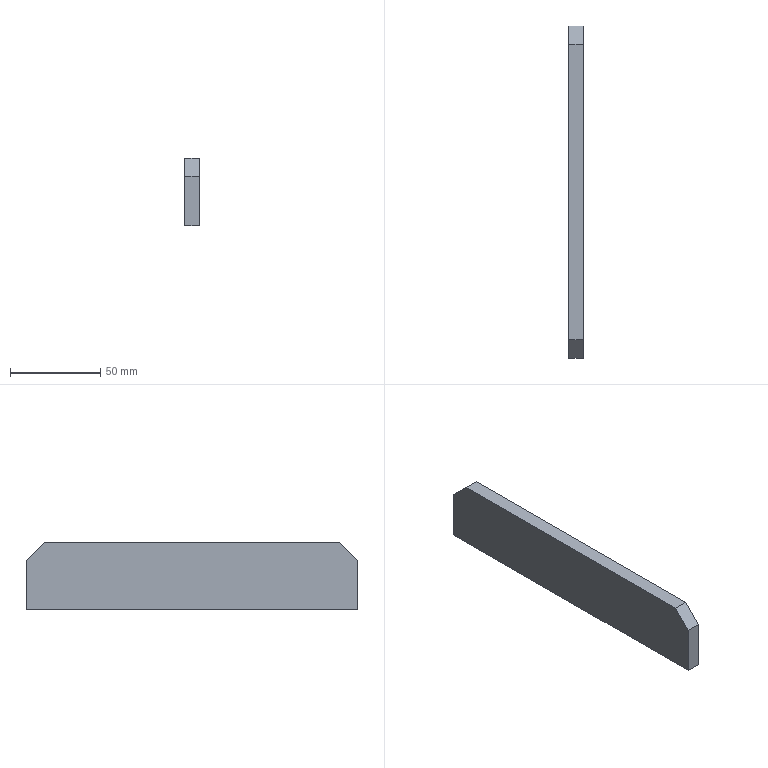Part | STEP file | Beam填充筋Plate-200×100 | 1 solid | 8 faces | box 8 x 184 x 37.25 mm | volume 54032 mm3 | plane 8
STEP:
#1=CARTESIAN_POINT('',(0.,0.,0.));
#2=DIRECTION('',(0.,0.,1.));
#3=DIRECTION('',(1.,0.,0.));
#4=AXIS2_PLACEMENT_3D('',#1,#2,#3);
#5=CARTESIAN_POINT('',(-4.,-92.,-18.625));
#6=VERTEX_POINT('',#5);
#7=CARTESIAN_POINT('',(-4.,92.,-18.625));
#8=VERTEX_POINT('',#7);
#9=CARTESIAN_POINT('',(-4.,92.,-18.625));
#10=DIRECTION('',(0.,1.,0.));
#11=VECTOR('',#10,1.);
#12=LINE('',#9,#11);
#13=CARTESIAN_POINT('',(4.,92.,-18.625));
#14=DIRECTION('',(0.,0.,1.));
#15=DIRECTION('',(0.,-1.,0.));
#16=AXIS2_PLACEMENT_3D('',#13,#14,#15);
#17=PLANE('',#16);
#18=CARTESIAN_POINT('',(0.,-8.));
#19=DIRECTION('',(-1.,0.));
#20=VECTOR('',#19,1.);
#21=LINE('',#18,#20);
#22=(GEOMETRIC_REPRESENTATION_CONTEXT(2)PARAMETRIC_REPRESENTATION_CONTEXT()REPRESENTATION_CONTEXT('',''));
#23=DEFINITIONAL_REPRESENTATION('',(#21),#22);
#24=PCURVE('',#17,#23);
#25=CARTESIAN_POINT('',(-4.,0.,0.));
#26=DIRECTION('',(1.,0.,0.));
#27=DIRECTION('',(0.,0.,-1.));
#28=AXIS2_PLACEMENT_3D('',#25,#26,#27);
#29=PLANE('',#28);
#30=CARTESIAN_POINT('',(18.625,92.));
#31=DIRECTION('',(0.,1.));
#32=VECTOR('',#31,1.);
#33=LINE('',#30,#32);
#34=(GEOMETRIC_REPRESENTATION_CONTEXT(2)PARAMETRIC_REPRESENTATION_CONTEXT()REPRESENTATION_CONTEXT('',''));
#35=DEFINITIONAL_REPRESENTATION('',(#33),#34);
#36=PCURVE('',#29,#35);
#37=SURFACE_CURVE('',#12,(#24,#36),.PCURVE_S1.);
#38=EDGE_CURVE('',#6,#8,#37,.T.);
#39=ORIENTED_EDGE('',*,*,#38,.T.);
#40=CARTESIAN_POINT('',(4.,92.,-18.625));
#41=VERTEX_POINT('',#40);
#42=CARTESIAN_POINT('',(4.,92.,-18.625));
#43=DIRECTION('',(-1.,0.,0.));
#44=VECTOR('',#43,1.);
#45=LINE('',#42,#44);
#46=CARTESIAN_POINT('',(0.,0.));
#47=DIRECTION('',(0.,-1.));
#48=VECTOR('',#47,1.);
#49=LINE('',#46,#48);
#50=(GEOMETRIC_REPRESENTATION_CONTEXT(2)PARAMETRIC_REPRESENTATION_CONTEXT()REPRESENTATION_CONTEXT('',''));
#51=DEFINITIONAL_REPRESENTATION('',(#49),#50);
#52=PCURVE('',#17,#51);
#53=CARTESIAN_POINT('',(4.,92.,18.625));
#54=DIRECTION('',(0.,-1.,0.));
#55=DIRECTION('',(0.,0.,-1.));
#56=AXIS2_PLACEMENT_3D('',#53,#54,#55);
#57=PLANE('',#56);
#58=CARTESIAN_POINT('',(37.25,0.));
#59=DIRECTION('',(0.,-1.));
#60=VECTOR('',#59,1.);
#61=LINE('',#58,#60);
#62=(GEOMETRIC_REPRESENTATION_CONTEXT(2)PARAMETRIC_REPRESENTATION_CONTEXT()REPRESENTATION_CONTEXT('',''));
#63=DEFINITIONAL_REPRESENTATION('',(#61),#62);
#64=PCURVE('',#57,#63);
#65=SURFACE_CURVE('',#45,(#52,#64),.PCURVE_S1.);
#66=EDGE_CURVE('',#41,#8,#65,.T.);
#67=ORIENTED_EDGE('',*,*,#66,.F.);
#68=CARTESIAN_POINT('',(4.,-92.,-18.625));
#69=VERTEX_POINT('',#68);
#70=CARTESIAN_POINT('',(4.,92.,-18.625));
#71=DIRECTION('',(0.,1.,0.));
#72=VECTOR('',#71,1.);
#73=LINE('',#70,#72);
#74=CARTESIAN_POINT('',(0.,0.));
#75=DIRECTION('',(-1.,0.));
#76=VECTOR('',#75,1.);
#77=LINE('',#74,#76);
#78=(GEOMETRIC_REPRESENTATION_CONTEXT(2)PARAMETRIC_REPRESENTATION_CONTEXT()REPRESENTATION_CONTEXT('',''));
#79=DEFINITIONAL_REPRESENTATION('',(#77),#78);
#80=PCURVE('',#17,#79);
#81=CARTESIAN_POINT('',(4.,0.,0.));
#82=DIRECTION('',(1.,0.,0.));
#83=DIRECTION('',(0.,0.,-1.));
#84=AXIS2_PLACEMENT_3D('',#81,#82,#83);
#85=PLANE('',#84);
#86=CARTESIAN_POINT('',(18.625,92.));
#87=DIRECTION('',(0.,1.));
#88=VECTOR('',#87,1.);
#89=LINE('',#86,#88);
#90=(GEOMETRIC_REPRESENTATION_CONTEXT(2)PARAMETRIC_REPRESENTATION_CONTEXT()REPRESENTATION_CONTEXT('',''));
#91=DEFINITIONAL_REPRESENTATION('',(#89),#90);
#92=PCURVE('',#85,#91);
#93=SURFACE_CURVE('',#73,(#80,#92),.PCURVE_S1.);
#94=EDGE_CURVE('',#69,#41,#93,.T.);
#95=ORIENTED_EDGE('',*,*,#94,.F.);
#96=CARTESIAN_POINT('',(4.,-92.,-18.625));
#97=DIRECTION('',(-1.,0.,0.));
#98=VECTOR('',#97,1.);
#99=LINE('',#96,#98);
#100=CARTESIAN_POINT('',(184.,0.));
#101=DIRECTION('',(0.,-1.));
#102=VECTOR('',#101,1.);
#103=LINE('',#100,#102);
#104=(GEOMETRIC_REPRESENTATION_CONTEXT(2)PARAMETRIC_REPRESENTATION_CONTEXT()REPRESENTATION_CONTEXT('',''));
#105=DEFINITIONAL_REPRESENTATION('',(#103),#104);
#106=PCURVE('',#17,#105);
#107=CARTESIAN_POINT('',(4.,-92.,18.625));
#108=DIRECTION('',(0.,1.,0.));
#109=DIRECTION('',(0.,0.,1.));
#110=AXIS2_PLACEMENT_3D('',#107,#108,#109);
#111=PLANE('',#110);
#112=CARTESIAN_POINT('',(-37.25,0.));
#113=DIRECTION('',(0.,-1.));
#114=VECTOR('',#113,1.);
#115=LINE('',#112,#114);
#116=(GEOMETRIC_REPRESENTATION_CONTEXT(2)PARAMETRIC_REPRESENTATION_CONTEXT()REPRESENTATION_CONTEXT('',''));
#117=DEFINITIONAL_REPRESENTATION('',(#115),#116);
#118=PCURVE('',#111,#117);
#119=SURFACE_CURVE('',#99,(#106,#118),.PCURVE_S1.);
#120=EDGE_CURVE('',#69,#6,#119,.T.);
#121=ORIENTED_EDGE('',*,*,#120,.T.);
#122=EDGE_LOOP('',(#39,#67,#95,#121));
#123=FACE_BOUND('',#122,.T.);
#124=ADVANCED_FACE('',(#123),#17,.F.);
#125=CARTESIAN_POINT('',(-4.,92.,8.625));
#126=VERTEX_POINT('',#125);
#127=CARTESIAN_POINT('',(-4.,92.,18.625));
#128=DIRECTION('',(0.,0.,1.));
#129=VECTOR('',#128,1.);
#130=LINE('',#127,#129);
#131=CARTESIAN_POINT('',(0.,-8.));
#132=DIRECTION('',(-1.,0.));
#133=VECTOR('',#132,1.);
#134=LINE('',#131,#133);
#135=(GEOMETRIC_REPRESENTATION_CONTEXT(2)PARAMETRIC_REPRESENTATION_CONTEXT()REPRESENTATION_CONTEXT('',''));
#136=DEFINITIONAL_REPRESENTATION('',(#134),#135);
#137=PCURVE('',#57,#136);
#138=CARTESIAN_POINT('',(-18.625,92.));
#139=DIRECTION('',(-1.,0.));
#140=VECTOR('',#139,1.);
#141=LINE('',#138,#140);
#142=(GEOMETRIC_REPRESENTATION_CONTEXT(2)PARAMETRIC_REPRESENTATION_CONTEXT()REPRESENTATION_CONTEXT('',''));
#143=DEFINITIONAL_REPRESENTATION('',(#141),#142);
#144=PCURVE('',#29,#143);
#145=SURFACE_CURVE('',#130,(#137,#144),.PCURVE_S1.);
#146=EDGE_CURVE('',#8,#126,#145,.T.);
#147=ORIENTED_EDGE('',*,*,#146,.T.);
#148=CARTESIAN_POINT('',(4.,92.,8.625));
#149=VERTEX_POINT('',#148);
#150=CARTESIAN_POINT('',(4.,92.,8.625));
#151=DIRECTION('',(1.,0.,0.));
#152=VECTOR('',#151,1.);
#153=LINE('',#150,#152);
#154=CARTESIAN_POINT('',(10.,0.));
#155=DIRECTION('',(0.,1.));
#156=VECTOR('',#155,1.);
#157=LINE('',#154,#156);
#158=(GEOMETRIC_REPRESENTATION_CONTEXT(2)PARAMETRIC_REPRESENTATION_CONTEXT()REPRESENTATION_CONTEXT('',''));
#159=DEFINITIONAL_REPRESENTATION('',(#157),#158);
#160=PCURVE('',#57,#159);
#161=CARTESIAN_POINT('',(4.,82.,18.625));
#162=DIRECTION('',(0.,-0.7071,-0.7071));
#163=DIRECTION('',(-1.,0.,0.));
#164=AXIS2_PLACEMENT_3D('',#161,#162,#163);
#165=PLANE('',#164);
#166=CARTESIAN_POINT('',(0.,14.142));
#167=DIRECTION('',(-1.,0.));
#168=VECTOR('',#167,1.);
#169=LINE('',#166,#168);
#170=(GEOMETRIC_REPRESENTATION_CONTEXT(2)PARAMETRIC_REPRESENTATION_CONTEXT()REPRESENTATION_CONTEXT('',''));
#171=DEFINITIONAL_REPRESENTATION('',(#169),#170);
#172=PCURVE('',#165,#171);
#173=SURFACE_CURVE('',#153,(#160,#172),.PCURVE_S1.);
#174=EDGE_CURVE('',#126,#149,#173,.T.);
#175=ORIENTED_EDGE('',*,*,#174,.T.);
#176=CARTESIAN_POINT('',(4.,92.,18.625));
#177=DIRECTION('',(0.,0.,1.));
#178=VECTOR('',#177,1.);
#179=LINE('',#176,#178);
#180=CARTESIAN_POINT('',(0.,0.));
#181=DIRECTION('',(-1.,0.));
#182=VECTOR('',#181,1.);
#183=LINE('',#180,#182);
#184=(GEOMETRIC_REPRESENTATION_CONTEXT(2)PARAMETRIC_REPRESENTATION_CONTEXT()REPRESENTATION_CONTEXT('',''));
#185=DEFINITIONAL_REPRESENTATION('',(#183),#184);
#186=PCURVE('',#57,#185);
#187=CARTESIAN_POINT('',(-18.625,92.));
#188=DIRECTION('',(-1.,0.));
#189=VECTOR('',#188,1.);
#190=LINE('',#187,#189);
#191=(GEOMETRIC_REPRESENTATION_CONTEXT(2)PARAMETRIC_REPRESENTATION_CONTEXT()REPRESENTATION_CONTEXT('',''));
#192=DEFINITIONAL_REPRESENTATION('',(#190),#191);
#193=PCURVE('',#85,#192);
#194=SURFACE_CURVE('',#179,(#186,#193),.PCURVE_S1.);
#195=EDGE_CURVE('',#41,#149,#194,.T.);
#196=ORIENTED_EDGE('',*,*,#195,.F.);
#197=ORIENTED_EDGE('',*,*,#66,.T.);
#198=EDGE_LOOP('',(#147,#175,#196,#197));
#199=FACE_BOUND('',#198,.T.);
#200=ADVANCED_FACE('',(#199),#57,.F.);
#201=CARTESIAN_POINT('',(-4.,82.,18.625));
#202=VERTEX_POINT('',#201);
#203=CARTESIAN_POINT('',(-4.,-82.,18.625));
#204=VERTEX_POINT('',#203);
#205=CARTESIAN_POINT('',(-4.,92.,18.625));
#206=DIRECTION('',(0.,-1.,0.));
#207=VECTOR('',#206,1.);
#208=LINE('',#205,#207);
#209=CARTESIAN_POINT('',(4.,92.,18.625));
#210=DIRECTION('',(0.,0.,-1.));
#211=DIRECTION('',(0.,1.,0.));
#212=AXIS2_PLACEMENT_3D('',#209,#210,#211);
#213=PLANE('',#212);
#214=CARTESIAN_POINT('',(0.,-8.));
#215=DIRECTION('',(-1.,0.));
#216=VECTOR('',#215,1.);
#217=LINE('',#214,#216);
#218=(GEOMETRIC_REPRESENTATION_CONTEXT(2)PARAMETRIC_REPRESENTATION_CONTEXT()REPRESENTATION_CONTEXT('',''));
#219=DEFINITIONAL_REPRESENTATION('',(#217),#218);
#220=PCURVE('',#213,#219);
#221=CARTESIAN_POINT('',(-18.625,92.));
#222=DIRECTION('',(0.,-1.));
#223=VECTOR('',#222,1.);
#224=LINE('',#221,#223);
#225=(GEOMETRIC_REPRESENTATION_CONTEXT(2)PARAMETRIC_REPRESENTATION_CONTEXT()REPRESENTATION_CONTEXT('',''));
#226=DEFINITIONAL_REPRESENTATION('',(#224),#225);
#227=PCURVE('',#29,#226);
#228=SURFACE_CURVE('',#208,(#220,#227),.PCURVE_S1.);
#229=EDGE_CURVE('',#202,#204,#228,.T.);
#230=ORIENTED_EDGE('',*,*,#229,.T.);
#231=CARTESIAN_POINT('',(4.,-82.,18.625));
#232=VERTEX_POINT('',#231);
#233=CARTESIAN_POINT('',(4.,-82.,18.625));
#234=DIRECTION('',(1.,0.,0.));
#235=VECTOR('',#234,1.);
#236=LINE('',#233,#235);
#237=CARTESIAN_POINT('',(-174.,0.));
#238=DIRECTION('',(0.,1.));
#239=VECTOR('',#238,1.);
#240=LINE('',#237,#239);
#241=(GEOMETRIC_REPRESENTATION_CONTEXT(2)PARAMETRIC_REPRESENTATION_CONTEXT()REPRESENTATION_CONTEXT('',''));
#242=DEFINITIONAL_REPRESENTATION('',(#240),#241);
#243=PCURVE('',#213,#242);
#244=CARTESIAN_POINT('',(4.,-92.,8.625));
#245=DIRECTION('',(0.,0.7071,-0.7071));
#246=DIRECTION('',(-1.,0.,0.));
#247=AXIS2_PLACEMENT_3D('',#244,#245,#246);
#248=PLANE('',#247);
#249=CARTESIAN_POINT('',(0.,14.142));
#250=DIRECTION('',(-1.,0.));
#251=VECTOR('',#250,1.);
#252=LINE('',#249,#251);
#253=(GEOMETRIC_REPRESENTATION_CONTEXT(2)PARAMETRIC_REPRESENTATION_CONTEXT()REPRESENTATION_CONTEXT('',''));
#254=DEFINITIONAL_REPRESENTATION('',(#252),#253);
#255=PCURVE('',#248,#254);
#256=SURFACE_CURVE('',#236,(#243,#255),.PCURVE_S1.);
#257=EDGE_CURVE('',#204,#232,#256,.T.);
#258=ORIENTED_EDGE('',*,*,#257,.T.);
#259=CARTESIAN_POINT('',(4.,82.,18.625));
#260=VERTEX_POINT('',#259);
#261=CARTESIAN_POINT('',(4.,92.,18.625));
#262=DIRECTION('',(0.,-1.,0.));
#263=VECTOR('',#262,1.);
#264=LINE('',#261,#263);
#265=CARTESIAN_POINT('',(0.,0.));
#266=DIRECTION('',(-1.,0.));
#267=VECTOR('',#266,1.);
#268=LINE('',#265,#267);
#269=(GEOMETRIC_REPRESENTATION_CONTEXT(2)PARAMETRIC_REPRESENTATION_CONTEXT()REPRESENTATION_CONTEXT('',''));
#270=DEFINITIONAL_REPRESENTATION('',(#268),#269);
#271=PCURVE('',#213,#270);
#272=CARTESIAN_POINT('',(-18.625,92.));
#273=DIRECTION('',(0.,-1.));
#274=VECTOR('',#273,1.);
#275=LINE('',#272,#274);
#276=(GEOMETRIC_REPRESENTATION_CONTEXT(2)PARAMETRIC_REPRESENTATION_CONTEXT()REPRESENTATION_CONTEXT('',''));
#277=DEFINITIONAL_REPRESENTATION('',(#275),#276);
#278=PCURVE('',#85,#277);
#279=SURFACE_CURVE('',#264,(#271,#278),.PCURVE_S1.);
#280=EDGE_CURVE('',#260,#232,#279,.T.);
#281=ORIENTED_EDGE('',*,*,#280,.F.);
#282=CARTESIAN_POINT('',(4.,82.,18.625));
#283=DIRECTION('',(-1.,0.,0.));
#284=VECTOR('',#283,1.);
#285=LINE('',#282,#284);
#286=CARTESIAN_POINT('',(-10.,0.));
#287=DIRECTION('',(0.,-1.));
#288=VECTOR('',#287,1.);
#289=LINE('',#286,#288);
#290=(GEOMETRIC_REPRESENTATION_CONTEXT(2)PARAMETRIC_REPRESENTATION_CONTEXT()REPRESENTATION_CONTEXT('',''));
#291=DEFINITIONAL_REPRESENTATION('',(#289),#290);
#292=PCURVE('',#213,#291);
#293=CARTESIAN_POINT('',(0.,0.));
#294=DIRECTION('',(1.,0.));
#295=VECTOR('',#294,1.);
#296=LINE('',#293,#295);
#297=(GEOMETRIC_REPRESENTATION_CONTEXT(2)PARAMETRIC_REPRESENTATION_CONTEXT()REPRESENTATION_CONTEXT('',''));
#298=DEFINITIONAL_REPRESENTATION('',(#296),#297);
#299=PCURVE('',#165,#298);
#300=SURFACE_CURVE('',#285,(#292,#299),.PCURVE_S1.);
#301=EDGE_CURVE('',#260,#202,#300,.T.);
#302=ORIENTED_EDGE('',*,*,#301,.T.);
#303=EDGE_LOOP('',(#230,#258,#281,#302));
#304=FACE_BOUND('',#303,.T.);
#305=ADVANCED_FACE('',(#304),#213,.F.);
#306=CARTESIAN_POINT('',(4.,-92.,8.625));
#307=VERTEX_POINT('',#306);
#308=CARTESIAN_POINT('',(4.,-92.,18.625));
#309=DIRECTION('',(0.,0.,-1.));
#310=VECTOR('',#309,1.);
#311=LINE('',#308,#310);
#312=CARTESIAN_POINT('',(0.,0.));
#313=DIRECTION('',(-1.,0.));
#314=VECTOR('',#313,1.);
#315=LINE('',#312,#314);
#316=(GEOMETRIC_REPRESENTATION_CONTEXT(2)PARAMETRIC_REPRESENTATION_CONTEXT()REPRESENTATION_CONTEXT('',''));
#317=DEFINITIONAL_REPRESENTATION('',(#315),#316);
#318=PCURVE('',#111,#317);
#319=CARTESIAN_POINT('',(-18.625,-92.));
#320=DIRECTION('',(1.,0.));
#321=VECTOR('',#320,1.);
#322=LINE('',#319,#321);
#323=(GEOMETRIC_REPRESENTATION_CONTEXT(2)PARAMETRIC_REPRESENTATION_CONTEXT()REPRESENTATION_CONTEXT('',''));
#324=DEFINITIONAL_REPRESENTATION('',(#322),#323);
#325=PCURVE('',#85,#324);
#326=SURFACE_CURVE('',#311,(#318,#325),.PCURVE_S1.);
#327=EDGE_CURVE('',#307,#69,#326,.T.);
#328=ORIENTED_EDGE('',*,*,#327,.F.);
#329=CARTESIAN_POINT('',(-4.,-92.,8.625));
#330=VERTEX_POINT('',#329);
#331=CARTESIAN_POINT('',(4.,-92.,8.625));
#332=DIRECTION('',(-1.,0.,0.));
#333=VECTOR('',#332,1.);
#334=LINE('',#331,#333);
#335=CARTESIAN_POINT('',(-10.,0.));
#336=DIRECTION('',(0.,-1.));
#337=VECTOR('',#336,1.);
#338=LINE('',#335,#337);
#339=(GEOMETRIC_REPRESENTATION_CONTEXT(2)PARAMETRIC_REPRESENTATION_CONTEXT()REPRESENTATION_CONTEXT('',''));
#340=DEFINITIONAL_REPRESENTATION('',(#338),#339);
#341=PCURVE('',#111,#340);
#342=CARTESIAN_POINT('',(0.,0.));
#343=DIRECTION('',(1.,0.));
#344=VECTOR('',#343,1.);
#345=LINE('',#342,#344);
#346=(GEOMETRIC_REPRESENTATION_CONTEXT(2)PARAMETRIC_REPRESENTATION_CONTEXT()REPRESENTATION_CONTEXT('',''));
#347=DEFINITIONAL_REPRESENTATION('',(#345),#346);
#348=PCURVE('',#248,#347);
#349=SURFACE_CURVE('',#334,(#341,#348),.PCURVE_S1.);
#350=EDGE_CURVE('',#307,#330,#349,.T.);
#351=ORIENTED_EDGE('',*,*,#350,.T.);
#352=CARTESIAN_POINT('',(-4.,-92.,18.625));
#353=DIRECTION('',(0.,0.,-1.));
#354=VECTOR('',#353,1.);
#355=LINE('',#352,#354);
#356=CARTESIAN_POINT('',(0.,-8.));
#357=DIRECTION('',(-1.,0.));
#358=VECTOR('',#357,1.);
#359=LINE('',#356,#358);
#360=(GEOMETRIC_REPRESENTATION_CONTEXT(2)PARAMETRIC_REPRESENTATION_CONTEXT()REPRESENTATION_CONTEXT('',''));
#361=DEFINITIONAL_REPRESENTATION('',(#359),#360);
#362=PCURVE('',#111,#361);
#363=CARTESIAN_POINT('',(-18.625,-92.));
#364=DIRECTION('',(1.,0.));
#365=VECTOR('',#364,1.);
#366=LINE('',#363,#365);
#367=(GEOMETRIC_REPRESENTATION_CONTEXT(2)PARAMETRIC_REPRESENTATION_CONTEXT()REPRESENTATION_CONTEXT('',''));
#368=DEFINITIONAL_REPRESENTATION('',(#366),#367);
#369=PCURVE('',#29,#368);
#370=SURFACE_CURVE('',#355,(#362,#369),.PCURVE_S1.);
#371=EDGE_CURVE('',#330,#6,#370,.T.);
#372=ORIENTED_EDGE('',*,*,#371,.T.);
#373=ORIENTED_EDGE('',*,*,#120,.F.);
#374=EDGE_LOOP('',(#328,#351,#372,#373));
#375=FACE_BOUND('',#374,.T.);
#376=ADVANCED_FACE('',(#375),#111,.F.);
#377=ORIENTED_EDGE('',*,*,#280,.T.);
#378=CARTESIAN_POINT('',(4.,-50.312,50.312));
#379=DIRECTION('',(0.,-0.7071,-0.7071));
#380=VECTOR('',#379,1.);
#381=LINE('',#378,#380);
#382=CARTESIAN_POINT('',(-50.312,-50.312));
#383=DIRECTION('',(0.7071,-0.7071));
#384=VECTOR('',#383,1.);
#385=LINE('',#382,#384);
#386=(GEOMETRIC_REPRESENTATION_CONTEXT(2)PARAMETRIC_REPRESENTATION_CONTEXT()REPRESENTATION_CONTEXT('',''));
#387=DEFINITIONAL_REPRESENTATION('',(#385),#386);
#388=PCURVE('',#85,#387);
#389=CARTESIAN_POINT('',(0.,58.955));
#390=DIRECTION('',(0.,-1.));
#391=VECTOR('',#390,1.);
#392=LINE('',#389,#391);
#393=(GEOMETRIC_REPRESENTATION_CONTEXT(2)PARAMETRIC_REPRESENTATION_CONTEXT()REPRESENTATION_CONTEXT('',''));
#394=DEFINITIONAL_REPRESENTATION('',(#392),#393);
#395=PCURVE('',#248,#394);
#396=SURFACE_CURVE('',#381,(#388,#395),.PCURVE_S1.);
#397=EDGE_CURVE('',#232,#307,#396,.T.);
#398=ORIENTED_EDGE('',*,*,#397,.T.);
#399=ORIENTED_EDGE('',*,*,#327,.T.);
#400=ORIENTED_EDGE('',*,*,#94,.T.);
#401=ORIENTED_EDGE('',*,*,#195,.T.);
#402=CARTESIAN_POINT('',(4.,50.312,50.312));
#403=DIRECTION('',(0.,-0.7071,0.7071));
#404=VECTOR('',#403,1.);
#405=LINE('',#402,#404);
#406=CARTESIAN_POINT('',(-50.312,50.312));
#407=DIRECTION('',(-0.7071,-0.7071));
#408=VECTOR('',#407,1.);
#409=LINE('',#406,#408);
#410=(GEOMETRIC_REPRESENTATION_CONTEXT(2)PARAMETRIC_REPRESENTATION_CONTEXT()REPRESENTATION_CONTEXT('',''));
#411=DEFINITIONAL_REPRESENTATION('',(#409),#410);
#412=PCURVE('',#85,#411);
#413=CARTESIAN_POINT('',(0.,-44.813));
#414=DIRECTION('',(0.,-1.));
#415=VECTOR('',#414,1.);
#416=LINE('',#413,#415);
#417=(GEOMETRIC_REPRESENTATION_CONTEXT(2)PARAMETRIC_REPRESENTATION_CONTEXT()REPRESENTATION_CONTEXT('',''));
#418=DEFINITIONAL_REPRESENTATION('',(#416),#417);
#419=PCURVE('',#165,#418);
#420=SURFACE_CURVE('',#405,(#412,#419),.PCURVE_S1.);
#421=EDGE_CURVE('',#149,#260,#420,.T.);
#422=ORIENTED_EDGE('',*,*,#421,.T.);
#423=EDGE_LOOP('',(#377,#398,#399,#400,#401,#422));
#424=FACE_BOUND('',#423,.T.);
#425=ADVANCED_FACE('',(#424),#85,.T.);
#426=ORIENTED_EDGE('',*,*,#371,.F.);
#427=CARTESIAN_POINT('',(-4.,-92.,8.625));
#428=DIRECTION('',(0.,0.7071,0.7071));
#429=VECTOR('',#428,1.);
#430=LINE('',#427,#429);
#431=CARTESIAN_POINT('',(-8.625,-92.));
#432=DIRECTION('',(-0.7071,0.7071));
#433=VECTOR('',#432,1.);
#434=LINE('',#431,#433);
#435=(GEOMETRIC_REPRESENTATION_CONTEXT(2)PARAMETRIC_REPRESENTATION_CONTEXT()REPRESENTATION_CONTEXT('',''));
#436=DEFINITIONAL_REPRESENTATION('',(#434),#435);
#437=PCURVE('',#29,#436);
#438=CARTESIAN_POINT('',(8.,0.));
#439=DIRECTION('',(0.,1.));
#440=VECTOR('',#439,1.);
#441=LINE('',#438,#440);
#442=(GEOMETRIC_REPRESENTATION_CONTEXT(2)PARAMETRIC_REPRESENTATION_CONTEXT()REPRESENTATION_CONTEXT('',''));
#443=DEFINITIONAL_REPRESENTATION('',(#441),#442);
#444=PCURVE('',#248,#443);
#445=SURFACE_CURVE('',#430,(#437,#444),.PCURVE_S1.);
#446=EDGE_CURVE('',#330,#204,#445,.T.);
#447=ORIENTED_EDGE('',*,*,#446,.T.);
#448=ORIENTED_EDGE('',*,*,#229,.F.);
#449=CARTESIAN_POINT('',(-4.,82.,18.625));
#450=DIRECTION('',(0.,0.7071,-0.7071));
#451=VECTOR('',#450,1.);
#452=LINE('',#449,#451);
#453=CARTESIAN_POINT('',(-18.625,82.));
#454=DIRECTION('',(0.7071,0.7071));
#455=VECTOR('',#454,1.);
#456=LINE('',#453,#455);
#457=(GEOMETRIC_REPRESENTATION_CONTEXT(2)PARAMETRIC_REPRESENTATION_CONTEXT()REPRESENTATION_CONTEXT('',''));
#458=DEFINITIONAL_REPRESENTATION('',(#456),#457);
#459=PCURVE('',#29,#458);
#460=CARTESIAN_POINT('',(8.,0.));
#461=DIRECTION('',(0.,1.));
#462=VECTOR('',#461,1.);
#463=LINE('',#460,#462);
#464=(GEOMETRIC_REPRESENTATION_CONTEXT(2)PARAMETRIC_REPRESENTATION_CONTEXT()REPRESENTATION_CONTEXT('',''));
#465=DEFINITIONAL_REPRESENTATION('',(#463),#464);
#466=PCURVE('',#165,#465);
#467=SURFACE_CURVE('',#452,(#459,#466),.PCURVE_S1.);
#468=EDGE_CURVE('',#202,#126,#467,.T.);
#469=ORIENTED_EDGE('',*,*,#468,.T.);
#470=ORIENTED_EDGE('',*,*,#146,.F.);
#471=ORIENTED_EDGE('',*,*,#38,.F.);
#472=EDGE_LOOP('',(#426,#447,#448,#469,#470,#471));
#473=FACE_BOUND('',#472,.T.);
#474=ADVANCED_FACE('',(#473),#29,.F.);
#475=ORIENTED_EDGE('',*,*,#397,.F.);
#476=ORIENTED_EDGE('',*,*,#257,.F.);
#477=ORIENTED_EDGE('',*,*,#446,.F.);
#478=ORIENTED_EDGE('',*,*,#350,.F.);
#479=EDGE_LOOP('',(#475,#476,#477,#478));
#480=FACE_BOUND('',#479,.T.);
#481=ADVANCED_FACE('',(#480),#248,.F.);
#482=ORIENTED_EDGE('',*,*,#421,.F.);
#483=ORIENTED_EDGE('',*,*,#174,.F.);
#484=ORIENTED_EDGE('',*,*,#468,.F.);
#485=ORIENTED_EDGE('',*,*,#301,.F.);
#486=EDGE_LOOP('',(#482,#483,#484,#485));
#487=FACE_BOUND('',#486,.T.);
#488=ADVANCED_FACE('',(#487),#165,.F.);
#489=CLOSED_SHELL('',(#124,#200,#305,#376,#425,#474,#481,#488));
#490=MANIFOLD_SOLID_BREP('',#489);
#491=(LENGTH_UNIT()NAMED_UNIT(*)SI_UNIT(.MILLI.,.METRE.));
#492=UNCERTAINTY_MEASURE_WITH_UNIT(LENGTH_MEASURE(0.0000001),#491,'','');
#493=(NAMED_UNIT(*)PLANE_ANGLE_UNIT()SI_UNIT($,.RADIAN.));
#494=(NAMED_UNIT(*)SI_UNIT($,.STERADIAN.)SOLID_ANGLE_UNIT());
#495=(GEOMETRIC_REPRESENTATION_CONTEXT(3)GLOBAL_UNCERTAINTY_ASSIGNED_CONTEXT((#492))GLOBAL_UNIT_ASSIGNED_CONTEXT((#491,#493,#494))REPRESENTATION_CONTEXT('',''));
#496=ADVANCED_BREP_SHAPE_REPRESENTATION('',(#4,#490),#495);